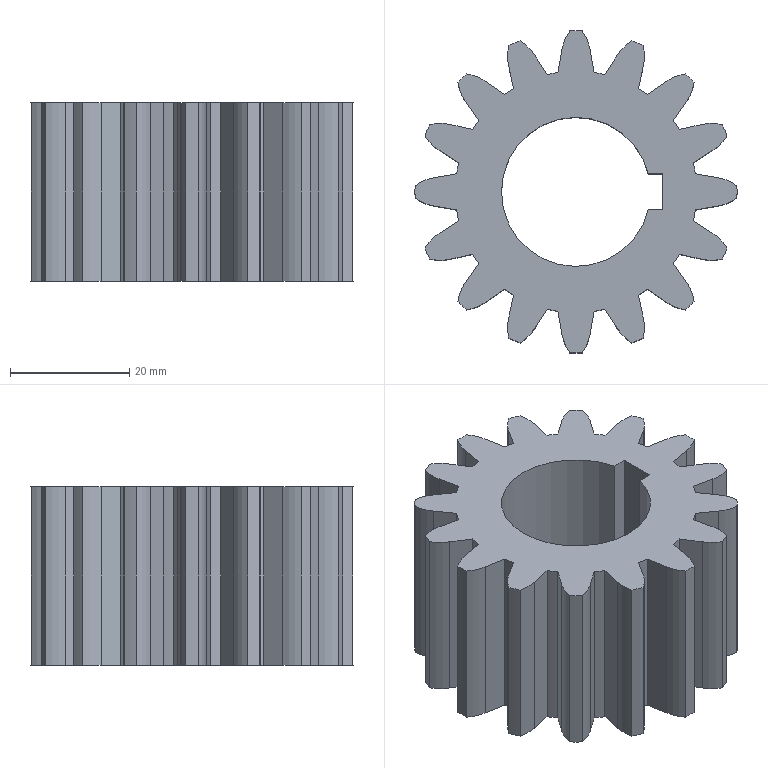Part | Creo | features PROTRUSION 17, DATUM PLANE 3, CURVE 2, COORDINATE SYSTEM 1, PATTERN 1 | 1 solid | 102 faces | box 54 x 54 x 30 mm | volume 38517 mm3 | cylinder 65 | plane 37 | commonest cylinder face diameters 14.705 x32 40.5 x16 54 x16 25 x1